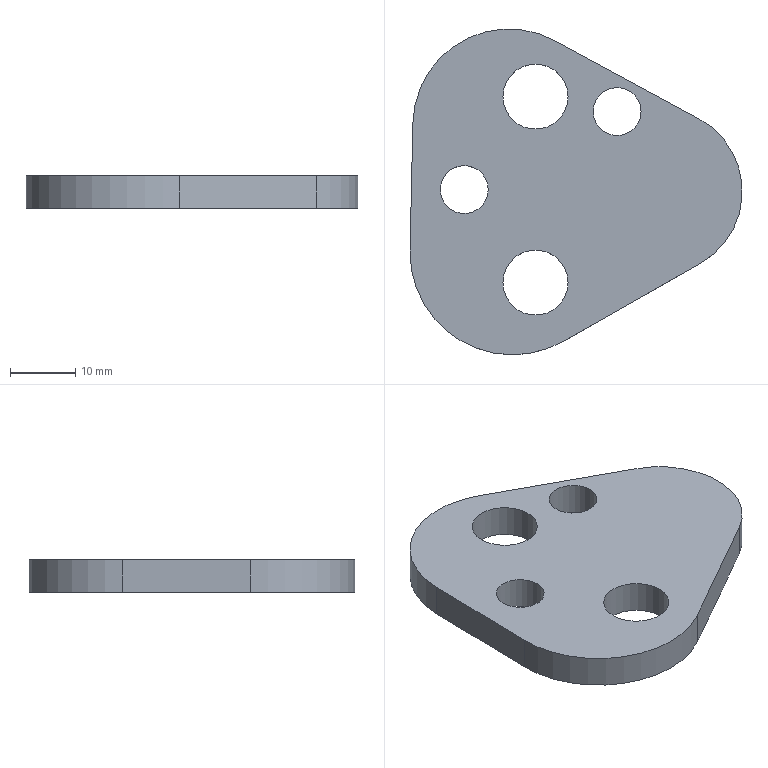Part | STEP file | 1_id198_x_t | 1 solid | 12 faces | box 51.017 x 50.028 x 5 mm | volume 8124 mm3 | cylinder 7 | plane 5 | commonest cylinder face diameters 7.35 x2 10 x2 25.4 x1 29.48 x1 31.48 x1
STEP:
#1=CARTESIAN_POINT('',(0.,0.,0.));
#2=DIRECTION('',(0.,0.,1.));
#3=DIRECTION('',(1.,0.,0.));
#4=AXIS2_PLACEMENT_3D('',#1,#2,#3);
#5=CARTESIAN_POINT('',(111.691,168.233,104.08));
#6=VERTEX_POINT('',#5);
#7=CARTESIAN_POINT('',(135.209,154.198,104.08));
#8=VERTEX_POINT('',#7);
#9=CARTESIAN_POINT('',(127.427,167.88,104.08));
#10=DIRECTION('',(0.,0.,1.));
#11=DIRECTION('',(-0.9997,0.02241,0.));
#12=AXIS2_PLACEMENT_3D('',#9,#10,#11);
#13=CIRCLE('',#12,15.74);
#14=CARTESIAN_POINT('',(127.427,167.88,109.08));
#15=DIRECTION('',(0.,0.,-1.));
#16=DIRECTION('',(1.,0.,0.));
#17=AXIS2_PLACEMENT_3D('',#14,#15,#16);
#18=CYLINDRICAL_SURFACE('',#17,15.74);
#19=CARTESIAN_POINT('',(9.447,5.));
#20=DIRECTION('',(-1.,0.));
#21=VECTOR('',#20,1.);
#22=LINE('',#19,#21);
#23=(GEOMETRIC_REPRESENTATION_CONTEXT(2)PARAMETRIC_REPRESENTATION_CONTEXT()REPRESENTATION_CONTEXT('',''));
#24=DEFINITIONAL_REPRESENTATION('',(#22),#23);
#25=PCURVE('',#18,#24);
#26=CARTESIAN_POINT('',(150.,177.5,104.08));
#27=DIRECTION('',(0.,0.,1.));
#28=DIRECTION('',(1.,0.,0.));
#29=AXIS2_PLACEMENT_3D('',#26,#27,#28);
#30=PLANE('',#29);
#31=CARTESIAN_POINT('',(-22.573,-9.62));
#32=DIRECTION('',(-0.9997,0.02241));
#33=AXIS2_PLACEMENT_2D('',#31,#32);
#34=CIRCLE('',#33,15.74);
#35=(GEOMETRIC_REPRESENTATION_CONTEXT(2)PARAMETRIC_REPRESENTATION_CONTEXT()REPRESENTATION_CONTEXT('',''));
#36=DEFINITIONAL_REPRESENTATION('',(#34),#35);
#37=PCURVE('',#30,#36);
#38=SURFACE_CURVE('',#13,(#25,#37),.PCURVE_S1.);
#39=EDGE_CURVE('',#6,#8,#38,.T.);
#40=ORIENTED_EDGE('',*,*,#39,.T.);
#41=CARTESIAN_POINT('',(135.209,154.198,109.08));
#42=VERTEX_POINT('',#41);
#43=CARTESIAN_POINT('',(135.209,154.198,104.08));
#44=DIRECTION('',(0.,0.,1.));
#45=VECTOR('',#44,1.);
#46=LINE('',#43,#45);
#47=CARTESIAN_POINT('',(1.054,5.));
#48=DIRECTION('',(0.,-1.));
#49=VECTOR('',#48,1.);
#50=LINE('',#47,#49);
#51=(GEOMETRIC_REPRESENTATION_CONTEXT(2)PARAMETRIC_REPRESENTATION_CONTEXT()REPRESENTATION_CONTEXT('',''));
#52=DEFINITIONAL_REPRESENTATION('',(#50),#51);
#53=PCURVE('',#18,#52);
#54=CARTESIAN_POINT('',(134.783,153.956,109.08));
#55=DIRECTION('',(-0.4944,0.8692,0.));
#56=DIRECTION('',(0.8692,0.4944,0.));
#57=AXIS2_PLACEMENT_3D('',#54,#55,#56);
#58=PLANE('',#57);
#59=CARTESIAN_POINT('',(0.4896,5.));
#60=DIRECTION('',(0.,-1.));
#61=VECTOR('',#60,1.);
#62=LINE('',#59,#61);
#63=(GEOMETRIC_REPRESENTATION_CONTEXT(2)PARAMETRIC_REPRESENTATION_CONTEXT()REPRESENTATION_CONTEXT('',''));
#64=DEFINITIONAL_REPRESENTATION('',(#62),#63);
#65=PCURVE('',#58,#64);
#66=SURFACE_CURVE('',#46,(#53,#65),.PCURVE_S1.);
#67=EDGE_CURVE('',#8,#42,#66,.T.);
#68=ORIENTED_EDGE('',*,*,#67,.T.);
#69=CARTESIAN_POINT('',(111.691,168.233,109.08));
#70=VERTEX_POINT('',#69);
#71=CARTESIAN_POINT('',(127.427,167.88,109.08));
#72=DIRECTION('',(0.,0.,-1.));
#73=DIRECTION('',(-1.,0.,0.));
#74=AXIS2_PLACEMENT_3D('',#71,#72,#73);
#75=CIRCLE('',#74,15.74);
#76=CARTESIAN_POINT('',(-3.142,0.));
#77=DIRECTION('',(1.,0.));
#78=VECTOR('',#77,1.);
#79=LINE('',#76,#78);
#80=(GEOMETRIC_REPRESENTATION_CONTEXT(2)PARAMETRIC_REPRESENTATION_CONTEXT()REPRESENTATION_CONTEXT('',''));
#81=DEFINITIONAL_REPRESENTATION('',(#79),#80);
#82=PCURVE('',#18,#81);
#83=CARTESIAN_POINT('',(150.,177.5,109.08));
#84=DIRECTION('',(0.,0.,1.));
#85=DIRECTION('',(1.,0.,0.));
#86=AXIS2_PLACEMENT_3D('',#83,#84,#85);
#87=PLANE('',#86);
#88=CARTESIAN_POINT('',(-38.313,-9.62));
#89=CARTESIAN_POINT('',(-38.313,17.643));
#90=CARTESIAN_POINT('',(-14.703,4.011));
#91=CARTESIAN_POINT('',(8.907,-9.62));
#92=CARTESIAN_POINT('',(-14.703,-23.251));
#93=CARTESIAN_POINT('',(-38.313,-36.882));
#94=CARTESIAN_POINT('',(-38.313,-9.62));
#95=(BOUNDED_CURVE()B_SPLINE_CURVE(2,(#88,#89,#90,#91,#92,#93,#94),.UNSPECIFIED.,.T.,.F.)B_SPLINE_CURVE_WITH_KNOTS((1,2,2,2,2,1),(-2.094,0.,2.094,4.189,6.283,8.378),.UNSPECIFIED.)CURVE()GEOMETRIC_REPRESENTATION_ITEM()RATIONAL_B_SPLINE_CURVE((1.,0.5,1.,0.5,1.,0.5,1.))REPRESENTATION_ITEM(''));
#96=(GEOMETRIC_REPRESENTATION_CONTEXT(2)PARAMETRIC_REPRESENTATION_CONTEXT()REPRESENTATION_CONTEXT('',''));
#97=DEFINITIONAL_REPRESENTATION('',(#95),#96);
#98=PCURVE('',#87,#97);
#99=SURFACE_CURVE('',#75,(#82,#98),.PCURVE_S1.);
#100=EDGE_CURVE('',#42,#70,#99,.T.);
#101=ORIENTED_EDGE('',*,*,#100,.T.);
#102=CARTESIAN_POINT('',(111.691,168.233,109.08));
#103=DIRECTION('',(0.,0.,-1.));
#104=VECTOR('',#103,1.);
#105=LINE('',#102,#104);
#106=CARTESIAN_POINT('',(3.164,0.));
#107=DIRECTION('',(0.,1.));
#108=VECTOR('',#107,1.);
#109=LINE('',#106,#108);
#110=(GEOMETRIC_REPRESENTATION_CONTEXT(2)PARAMETRIC_REPRESENTATION_CONTEXT()REPRESENTATION_CONTEXT('',''));
#111=DEFINITIONAL_REPRESENTATION('',(#109),#110);
#112=PCURVE('',#18,#111);
#113=CARTESIAN_POINT('',(112.118,187.28,109.08));
#114=DIRECTION('',(0.9997,-0.02241,0.));
#115=DIRECTION('',(0.,0.,1.));
#116=AXIS2_PLACEMENT_3D('',#113,#114,#115);
#117=PLANE('',#116);
#118=CARTESIAN_POINT('',(0.,19.052));
#119=DIRECTION('',(-1.,0.));
#120=VECTOR('',#119,1.);
#121=LINE('',#118,#120);
#122=(GEOMETRIC_REPRESENTATION_CONTEXT(2)PARAMETRIC_REPRESENTATION_CONTEXT()REPRESENTATION_CONTEXT('',''));
#123=DEFINITIONAL_REPRESENTATION('',(#121),#122);
#124=PCURVE('',#117,#123);
#125=SURFACE_CURVE('',#105,(#112,#124),.PCURVE_S1.);
#126=EDGE_CURVE('',#70,#6,#125,.T.);
#127=ORIENTED_EDGE('',*,*,#126,.T.);
#128=EDGE_LOOP('',(#40,#68,#101,#127));
#129=FACE_BOUND('',#128,.T.);
#130=ADVANCED_FACE('',(#129),#18,.T.);
#131=CARTESIAN_POINT('',(135.95,163.225,104.08));
#132=VERTEX_POINT('',#131);
#133=CARTESIAN_POINT('',(130.95,163.225,104.08));
#134=DIRECTION('',(0.,0.,1.));
#135=DIRECTION('',(1.,0.,0.));
#136=AXIS2_PLACEMENT_3D('',#133,#134,#135);
#137=CIRCLE('',#136,5.);
#138=CARTESIAN_POINT('',(-19.05,-14.275));
#139=DIRECTION('',(1.,0.));
#140=AXIS2_PLACEMENT_2D('',#138,#139);
#141=CIRCLE('',#140,5.);
#142=(GEOMETRIC_REPRESENTATION_CONTEXT(2)PARAMETRIC_REPRESENTATION_CONTEXT()REPRESENTATION_CONTEXT('',''));
#143=DEFINITIONAL_REPRESENTATION('',(#141),#142);
#144=PCURVE('',#30,#143);
#145=CARTESIAN_POINT('',(130.95,163.225,-109.08));
#146=DIRECTION('',(0.,0.,1.));
#147=DIRECTION('',(1.,0.,0.));
#148=AXIS2_PLACEMENT_3D('',#145,#146,#147);
#149=CYLINDRICAL_SURFACE('',#148,5.);
#150=CARTESIAN_POINT('',(0.,213.16));
#151=DIRECTION('',(1.,0.));
#152=VECTOR('',#151,1.);
#153=LINE('',#150,#152);
#154=(GEOMETRIC_REPRESENTATION_CONTEXT(2)PARAMETRIC_REPRESENTATION_CONTEXT()REPRESENTATION_CONTEXT('',''));
#155=DEFINITIONAL_REPRESENTATION('',(#153),#154);
#156=PCURVE('',#149,#155);
#157=SURFACE_CURVE('',#137,(#144,#156),.PCURVE_S1.);
#158=EDGE_CURVE('',#132,#132,#157,.T.);
#159=ORIENTED_EDGE('',*,*,#158,.T.);
#160=EDGE_LOOP('',(#159));
#161=FACE_BOUND('',#160,.T.);
#162=CARTESIAN_POINT('',(135.95,191.775,104.08));
#163=VERTEX_POINT('',#162);
#164=CARTESIAN_POINT('',(130.95,191.775,104.08));
#165=DIRECTION('',(0.,0.,1.));
#166=DIRECTION('',(1.,0.,0.));
#167=AXIS2_PLACEMENT_3D('',#164,#165,#166);
#168=CIRCLE('',#167,5.);
#169=CARTESIAN_POINT('',(-19.05,14.275));
#170=DIRECTION('',(1.,0.));
#171=AXIS2_PLACEMENT_2D('',#169,#170);
#172=CIRCLE('',#171,5.);
#173=(GEOMETRIC_REPRESENTATION_CONTEXT(2)PARAMETRIC_REPRESENTATION_CONTEXT()REPRESENTATION_CONTEXT('',''));
#174=DEFINITIONAL_REPRESENTATION('',(#172),#173);
#175=PCURVE('',#30,#174);
#176=CARTESIAN_POINT('',(130.95,191.775,-109.08));
#177=DIRECTION('',(0.,0.,1.));
#178=DIRECTION('',(1.,0.,0.));
#179=AXIS2_PLACEMENT_3D('',#176,#177,#178);
#180=CYLINDRICAL_SURFACE('',#179,5.);
#181=CARTESIAN_POINT('',(0.,213.16));
#182=DIRECTION('',(1.,0.));
#183=VECTOR('',#182,1.);
#184=LINE('',#181,#183);
#185=(GEOMETRIC_REPRESENTATION_CONTEXT(2)PARAMETRIC_REPRESENTATION_CONTEXT()REPRESENTATION_CONTEXT('',''));
#186=DEFINITIONAL_REPRESENTATION('',(#184),#185);
#187=PCURVE('',#180,#186);
#188=SURFACE_CURVE('',#168,(#175,#187),.PCURVE_S1.);
#189=EDGE_CURVE('',#163,#163,#188,.T.);
#190=ORIENTED_EDGE('',*,*,#189,.T.);
#191=EDGE_LOOP('',(#190));
#192=FACE_BOUND('',#191,.T.);
#193=ORIENTED_EDGE('',*,*,#39,.F.);
#194=CARTESIAN_POINT('',(112.129,187.758,104.08));
#195=VERTEX_POINT('',#194);
#196=CARTESIAN_POINT('',(111.918,178.354,104.08));
#197=DIRECTION('',(0.02241,0.9997,0.));
#198=VECTOR('',#197,1.);
#199=LINE('',#196,#198);
#200=CARTESIAN_POINT('',(-38.082,0.8537));
#201=DIRECTION('',(0.02241,0.9997));
#202=VECTOR('',#201,1.);
#203=LINE('',#200,#202);
#204=(GEOMETRIC_REPRESENTATION_CONTEXT(2)PARAMETRIC_REPRESENTATION_CONTEXT()REPRESENTATION_CONTEXT('',''));
#205=DEFINITIONAL_REPRESENTATION('',(#203),#204);
#206=PCURVE('',#30,#205);
#207=CARTESIAN_POINT('',(-5.,8.928));
#208=DIRECTION('',(0.,-1.));
#209=VECTOR('',#208,1.);
#210=LINE('',#207,#209);
#211=(GEOMETRIC_REPRESENTATION_CONTEXT(2)PARAMETRIC_REPRESENTATION_CONTEXT()REPRESENTATION_CONTEXT('',''));
#212=DEFINITIONAL_REPRESENTATION('',(#210),#211);
#213=PCURVE('',#117,#212);
#214=SURFACE_CURVE('',#199,(#206,#213),.PCURVE_S1.);
#215=EDGE_CURVE('',#6,#195,#214,.T.);
#216=ORIENTED_EDGE('',*,*,#215,.T.);
#217=CARTESIAN_POINT('',(133.881,200.391,104.08));
#218=VERTEX_POINT('',#217);
#219=CARTESIAN_POINT('',(126.865,187.428,104.08));
#220=DIRECTION('',(0.,0.,-1.));
#221=DIRECTION('',(-0.9997,0.02241,0.));
#222=AXIS2_PLACEMENT_3D('',#219,#220,#221);
#223=CIRCLE('',#222,14.74);
#224=CARTESIAN_POINT('',(-37.871,10.258));
#225=CARTESIAN_POINT('',(-37.299,35.782));
#226=CARTESIAN_POINT('',(-15.481,22.525));
#227=CARTESIAN_POINT('',(6.338,9.267));
#228=CARTESIAN_POINT('',(-16.053,-2.999));
#229=CARTESIAN_POINT('',(-38.444,-15.266));
#230=CARTESIAN_POINT('',(-37.871,10.258));
#231=(BOUNDED_CURVE()B_SPLINE_CURVE(2,(#224,#225,#226,#227,#228,#229,#230),.UNSPECIFIED.,.T.,.F.)B_SPLINE_CURVE_WITH_KNOTS((1,2,2,2,2,1),(-2.094,0.,2.094,4.189,6.283,8.378),.UNSPECIFIED.)CURVE()GEOMETRIC_REPRESENTATION_ITEM()RATIONAL_B_SPLINE_CURVE((1.,0.5,1.,0.5,1.,0.5,1.))REPRESENTATION_ITEM(''));
#232=(GEOMETRIC_REPRESENTATION_CONTEXT(2)PARAMETRIC_REPRESENTATION_CONTEXT()REPRESENTATION_CONTEXT('',''));
#233=DEFINITIONAL_REPRESENTATION('',(#231),#232);
#234=PCURVE('',#30,#233);
#235=CARTESIAN_POINT('',(126.865,187.428,109.08));
#236=DIRECTION('',(0.,0.,-1.));
#237=DIRECTION('',(1.,0.,0.));
#238=AXIS2_PLACEMENT_3D('',#235,#236,#237);
#239=CYLINDRICAL_SURFACE('',#238,14.74);
#240=CARTESIAN_POINT('',(3.164,5.));
#241=DIRECTION('',(1.,0.));
#242=VECTOR('',#241,1.);
#243=LINE('',#240,#242);
#244=(GEOMETRIC_REPRESENTATION_CONTEXT(2)PARAMETRIC_REPRESENTATION_CONTEXT()REPRESENTATION_CONTEXT('',''));
#245=DEFINITIONAL_REPRESENTATION('',(#243),#244);
#246=PCURVE('',#239,#245);
#247=SURFACE_CURVE('',#223,(#234,#246),.PCURVE_S1.);
#248=EDGE_CURVE('',#195,#218,#247,.T.);
#249=ORIENTED_EDGE('',*,*,#248,.T.);
#250=CARTESIAN_POINT('',(156.049,188.393,104.08));
#251=VERTEX_POINT('',#250);
#252=CARTESIAN_POINT('',(133.881,200.391,104.08));
#253=DIRECTION('',(0.8795,-0.476,0.));
#254=VECTOR('',#253,1.);
#255=LINE('',#252,#254);
#256=CARTESIAN_POINT('',(-16.119,22.891));
#257=DIRECTION('',(0.8795,-0.476));
#258=VECTOR('',#257,1.);
#259=LINE('',#256,#258);
#260=(GEOMETRIC_REPRESENTATION_CONTEXT(2)PARAMETRIC_REPRESENTATION_CONTEXT()REPRESENTATION_CONTEXT('',''));
#261=DEFINITIONAL_REPRESENTATION('',(#259),#260);
#262=PCURVE('',#30,#261);
#263=CARTESIAN_POINT('',(156.047,188.394,109.08));
#264=DIRECTION('',(-0.476,-0.8795,0.));
#265=DIRECTION('',(-0.8795,0.476,0.));
#266=AXIS2_PLACEMENT_3D('',#263,#264,#265);
#267=PLANE('',#266);
#268=CARTESIAN_POINT('',(25.205,5.));
#269=DIRECTION('',(-1.,0.));
#270=VECTOR('',#269,1.);
#271=LINE('',#268,#270);
#272=(GEOMETRIC_REPRESENTATION_CONTEXT(2)PARAMETRIC_REPRESENTATION_CONTEXT()REPRESENTATION_CONTEXT('',''));
#273=DEFINITIONAL_REPRESENTATION('',(#271),#272);
#274=PCURVE('',#267,#273);
#275=SURFACE_CURVE('',#255,(#262,#274),.PCURVE_S1.);
#276=EDGE_CURVE('',#218,#251,#275,.T.);
#277=ORIENTED_EDGE('',*,*,#276,.T.);
#278=CARTESIAN_POINT('',(156.283,166.185,104.08));
#279=VERTEX_POINT('',#278);
#280=CARTESIAN_POINT('',(150.004,177.224,104.08));
#281=DIRECTION('',(0.,0.,-1.));
#282=DIRECTION('',(1.,0.,0.));
#283=AXIS2_PLACEMENT_3D('',#280,#281,#282);
#284=CIRCLE('',#283,12.7);
#285=CARTESIAN_POINT('',(12.704,-0.2758));
#286=CARTESIAN_POINT('',(12.704,-22.273));
#287=CARTESIAN_POINT('',(-6.346,-11.274));
#288=CARTESIAN_POINT('',(-25.396,-0.2758));
#289=CARTESIAN_POINT('',(-6.346,10.723));
#290=CARTESIAN_POINT('',(12.704,21.721));
#291=CARTESIAN_POINT('',(12.704,-0.2758));
#292=(BOUNDED_CURVE()B_SPLINE_CURVE(2,(#285,#286,#287,#288,#289,#290,#291),.UNSPECIFIED.,.T.,.F.)B_SPLINE_CURVE_WITH_KNOTS((1,2,2,2,2,1),(-2.094,0.,2.094,4.189,6.283,8.378),.UNSPECIFIED.)CURVE()GEOMETRIC_REPRESENTATION_ITEM()RATIONAL_B_SPLINE_CURVE((1.,0.5,1.,0.5,1.,0.5,1.))REPRESENTATION_ITEM(''));
#293=(GEOMETRIC_REPRESENTATION_CONTEXT(2)PARAMETRIC_REPRESENTATION_CONTEXT()REPRESENTATION_CONTEXT('',''));
#294=DEFINITIONAL_REPRESENTATION('',(#292),#293);
#295=PCURVE('',#30,#294);
#296=CARTESIAN_POINT('',(150.004,177.224,109.08));
#297=DIRECTION('',(0.,0.,-1.));
#298=DIRECTION('',(1.,0.,0.));
#299=AXIS2_PLACEMENT_3D('',#296,#297,#298);
#300=CYLINDRICAL_SURFACE('',#299,12.7);
#301=CARTESIAN_POINT('',(0.,5.));
#302=DIRECTION('',(1.,0.));
#303=VECTOR('',#302,1.);
#304=LINE('',#301,#303);
#305=(GEOMETRIC_REPRESENTATION_CONTEXT(2)PARAMETRIC_REPRESENTATION_CONTEXT()REPRESENTATION_CONTEXT('',''));
#306=DEFINITIONAL_REPRESENTATION('',(#304),#305);
#307=PCURVE('',#300,#306);
#308=SURFACE_CURVE('',#284,(#295,#307),.PCURVE_S1.);
#309=EDGE_CURVE('',#251,#279,#308,.T.);
#310=ORIENTED_EDGE('',*,*,#309,.T.);
#311=CARTESIAN_POINT('',(156.283,166.185,104.08));
#312=DIRECTION('',(-0.8692,-0.4944,0.));
#313=VECTOR('',#312,1.);
#314=LINE('',#311,#313);
#315=CARTESIAN_POINT('',(6.283,-11.315));
#316=DIRECTION('',(-0.8692,-0.4944));
#317=VECTOR('',#316,1.);
#318=LINE('',#315,#317);
#319=(GEOMETRIC_REPRESENTATION_CONTEXT(2)PARAMETRIC_REPRESENTATION_CONTEXT()REPRESENTATION_CONTEXT('',''));
#320=DEFINITIONAL_REPRESENTATION('',(#318),#319);
#321=PCURVE('',#30,#320);
#322=CARTESIAN_POINT('',(24.734,5.));
#323=DIRECTION('',(-1.,0.));
#324=VECTOR('',#323,1.);
#325=LINE('',#322,#324);
#326=(GEOMETRIC_REPRESENTATION_CONTEXT(2)PARAMETRIC_REPRESENTATION_CONTEXT()REPRESENTATION_CONTEXT('',''));
#327=DEFINITIONAL_REPRESENTATION('',(#325),#326);
#328=PCURVE('',#58,#327);
#329=SURFACE_CURVE('',#314,(#321,#328),.PCURVE_S1.);
#330=EDGE_CURVE('',#279,#8,#329,.T.);
#331=ORIENTED_EDGE('',*,*,#330,.T.);
#332=EDGE_LOOP('',(#193,#216,#249,#277,#310,#331));
#333=FACE_BOUND('',#332,.T.);
#334=CARTESIAN_POINT('',(147.173,189.489,104.08));
#335=VERTEX_POINT('',#334);
#336=CARTESIAN_POINT('',(143.498,189.489,104.08));
#337=DIRECTION('',(0.,0.,1.));
#338=DIRECTION('',(1.,0.,0.));
#339=AXIS2_PLACEMENT_3D('',#336,#337,#338);
#340=CIRCLE('',#339,3.675);
#341=CARTESIAN_POINT('',(-6.502,11.989));
#342=DIRECTION('',(1.,0.));
#343=AXIS2_PLACEMENT_2D('',#341,#342);
#344=CIRCLE('',#343,3.675);
#345=(GEOMETRIC_REPRESENTATION_CONTEXT(2)PARAMETRIC_REPRESENTATION_CONTEXT()REPRESENTATION_CONTEXT('',''));
#346=DEFINITIONAL_REPRESENTATION('',(#344),#345);
#347=PCURVE('',#30,#346);
#348=CARTESIAN_POINT('',(143.498,189.489,109.08));
#349=DIRECTION('',(0.,0.,-1.));
#350=DIRECTION('',(1.,0.,0.));
#351=AXIS2_PLACEMENT_3D('',#348,#349,#350);
#352=CYLINDRICAL_SURFACE('',#351,3.675);
#353=CARTESIAN_POINT('',(6.283,5.));
#354=DIRECTION('',(-1.,0.));
#355=VECTOR('',#354,1.);
#356=LINE('',#353,#355);
#357=(GEOMETRIC_REPRESENTATION_CONTEXT(2)PARAMETRIC_REPRESENTATION_CONTEXT()REPRESENTATION_CONTEXT('',''));
#358=DEFINITIONAL_REPRESENTATION('',(#356),#357);
#359=PCURVE('',#352,#358);
#360=SURFACE_CURVE('',#340,(#347,#359),.PCURVE_S1.);
#361=EDGE_CURVE('',#335,#335,#360,.T.);
#362=ORIENTED_EDGE('',*,*,#361,.T.);
#363=EDGE_LOOP('',(#362));
#364=FACE_BOUND('',#363,.T.);
#365=CARTESIAN_POINT('',(123.703,177.5,104.08));
#366=VERTEX_POINT('',#365);
#367=CARTESIAN_POINT('',(120.028,177.5,104.08));
#368=DIRECTION('',(0.,0.,1.));
#369=DIRECTION('',(1.,0.,0.));
#370=AXIS2_PLACEMENT_3D('',#367,#368,#369);
#371=CIRCLE('',#370,3.675);
#372=CARTESIAN_POINT('',(-29.972,0.));
#373=DIRECTION('',(1.,0.));
#374=AXIS2_PLACEMENT_2D('',#372,#373);
#375=CIRCLE('',#374,3.675);
#376=(GEOMETRIC_REPRESENTATION_CONTEXT(2)PARAMETRIC_REPRESENTATION_CONTEXT()REPRESENTATION_CONTEXT('',''));
#377=DEFINITIONAL_REPRESENTATION('',(#375),#376);
#378=PCURVE('',#30,#377);
#379=CARTESIAN_POINT('',(120.028,177.5,109.08));
#380=DIRECTION('',(0.,0.,-1.));
#381=DIRECTION('',(1.,0.,0.));
#382=AXIS2_PLACEMENT_3D('',#379,#380,#381);
#383=CYLINDRICAL_SURFACE('',#382,3.675);
#384=CARTESIAN_POINT('',(6.283,5.));
#385=DIRECTION('',(-1.,0.));
#386=VECTOR('',#385,1.);
#387=LINE('',#384,#386);
#388=(GEOMETRIC_REPRESENTATION_CONTEXT(2)PARAMETRIC_REPRESENTATION_CONTEXT()REPRESENTATION_CONTEXT('',''));
#389=DEFINITIONAL_REPRESENTATION('',(#387),#388);
#390=PCURVE('',#383,#389);
#391=SURFACE_CURVE('',#371,(#378,#390),.PCURVE_S1.);
#392=EDGE_CURVE('',#366,#366,#391,.T.);
#393=ORIENTED_EDGE('',*,*,#392,.T.);
#394=EDGE_LOOP('',(#393));
#395=FACE_BOUND('',#394,.T.);
#396=ADVANCED_FACE('',(#161,#192,#333,#364,#395),#30,.F.);
#397=CARTESIAN_POINT('',(156.283,166.185,109.08));
#398=VERTEX_POINT('',#397);
#399=CARTESIAN_POINT('',(156.283,166.185,109.08));
#400=DIRECTION('',(0.,0.,-1.));
#401=VECTOR('',#400,1.);
#402=LINE('',#399,#401);
#403=CARTESIAN_POINT('',(24.734,0.));
#404=DIRECTION('',(0.,1.));
#405=VECTOR('',#404,1.);
#406=LINE('',#403,#405);
#407=(GEOMETRIC_REPRESENTATION_CONTEXT(2)PARAMETRIC_REPRESENTATION_CONTEXT()REPRESENTATION_CONTEXT('',''));
#408=DEFINITIONAL_REPRESENTATION('',(#406),#407);
#409=PCURVE('',#58,#408);
#410=CARTESIAN_POINT('',(7.337,0.));
#411=DIRECTION('',(0.,1.));
#412=VECTOR('',#411,1.);
#413=LINE('',#410,#412);
#414=(GEOMETRIC_REPRESENTATION_CONTEXT(2)PARAMETRIC_REPRESENTATION_CONTEXT()REPRESENTATION_CONTEXT('',''));
#415=DEFINITIONAL_REPRESENTATION('',(#413),#414);
#416=PCURVE('',#300,#415);
#417=SURFACE_CURVE('',#402,(#409,#416),.PCURVE_S1.);
#418=EDGE_CURVE('',#398,#279,#417,.T.);
#419=ORIENTED_EDGE('',*,*,#418,.F.);
#420=CARTESIAN_POINT('',(135.209,154.198,109.08));
#421=DIRECTION('',(0.8692,0.4944,0.));
#422=VECTOR('',#421,1.);
#423=LINE('',#420,#422);
#424=CARTESIAN_POINT('',(0.4896,0.));
#425=DIRECTION('',(1.,0.));
#426=VECTOR('',#425,1.);
#427=LINE('',#424,#426);
#428=(GEOMETRIC_REPRESENTATION_CONTEXT(2)PARAMETRIC_REPRESENTATION_CONTEXT()REPRESENTATION_CONTEXT('',''));
#429=DEFINITIONAL_REPRESENTATION('',(#427),#428);
#430=PCURVE('',#58,#429);
#431=CARTESIAN_POINT('',(-14.791,-23.302));
#432=DIRECTION('',(0.8692,0.4944));
#433=VECTOR('',#432,1.);
#434=LINE('',#431,#433);
#435=(GEOMETRIC_REPRESENTATION_CONTEXT(2)PARAMETRIC_REPRESENTATION_CONTEXT()REPRESENTATION_CONTEXT('',''));
#436=DEFINITIONAL_REPRESENTATION('',(#434),#435);
#437=PCURVE('',#87,#436);
#438=SURFACE_CURVE('',#423,(#430,#437),.PCURVE_S1.);
#439=EDGE_CURVE('',#42,#398,#438,.T.);
#440=ORIENTED_EDGE('',*,*,#439,.F.);
#441=ORIENTED_EDGE('',*,*,#67,.F.);
#442=ORIENTED_EDGE('',*,*,#330,.F.);
#443=EDGE_LOOP('',(#419,#440,#441,#442));
#444=FACE_BOUND('',#443,.T.);
#445=ADVANCED_FACE('',(#444),#58,.F.);
#446=CARTESIAN_POINT('',(135.95,163.225,109.08));
#447=VERTEX_POINT('',#446);
#448=CARTESIAN_POINT('',(130.95,163.225,109.08));
#449=DIRECTION('',(0.,0.,1.));
#450=DIRECTION('',(1.,0.,0.));
#451=AXIS2_PLACEMENT_3D('',#448,#449,#450);
#452=CIRCLE('',#451,5.);
#453=CARTESIAN_POINT('',(-19.05,-14.275));
#454=DIRECTION('',(1.,0.));
#455=AXIS2_PLACEMENT_2D('',#453,#454);
#456=CIRCLE('',#455,5.);
#457=(GEOMETRIC_REPRESENTATION_CONTEXT(2)PARAMETRIC_REPRESENTATION_CONTEXT()REPRESENTATION_CONTEXT('',''));
#458=DEFINITIONAL_REPRESENTATION('',(#456),#457);
#459=PCURVE('',#87,#458);
#460=CARTESIAN_POINT('',(0.,218.16));
#461=DIRECTION('',(1.,0.));
#462=VECTOR('',#461,1.);
#463=LINE('',#460,#462);
#464=(GEOMETRIC_REPRESENTATION_CONTEXT(2)PARAMETRIC_REPRESENTATION_CONTEXT()REPRESENTATION_CONTEXT('',''));
#465=DEFINITIONAL_REPRESENTATION('',(#463),#464);
#466=PCURVE('',#149,#465);
#467=SURFACE_CURVE('',#452,(#459,#466),.PCURVE_S1.);
#468=EDGE_CURVE('',#447,#447,#467,.T.);
#469=ORIENTED_EDGE('',*,*,#468,.F.);
#470=EDGE_LOOP('',(#469));
#471=FACE_BOUND('',#470,.T.);
#472=CARTESIAN_POINT('',(135.95,191.775,109.08));
#473=VERTEX_POINT('',#472);
#474=CARTESIAN_POINT('',(130.95,191.775,109.08));
#475=DIRECTION('',(0.,0.,1.));
#476=DIRECTION('',(1.,0.,0.));
#477=AXIS2_PLACEMENT_3D('',#474,#475,#476);
#478=CIRCLE('',#477,5.);
#479=CARTESIAN_POINT('',(-19.05,14.275));
#480=DIRECTION('',(1.,0.));
#481=AXIS2_PLACEMENT_2D('',#479,#480);
#482=CIRCLE('',#481,5.);
#483=(GEOMETRIC_REPRESENTATION_CONTEXT(2)PARAMETRIC_REPRESENTATION_CONTEXT()REPRESENTATION_CONTEXT('',''));
#484=DEFINITIONAL_REPRESENTATION('',(#482),#483);
#485=PCURVE('',#87,#484);
#486=CARTESIAN_POINT('',(0.,218.16));
#487=DIRECTION('',(1.,0.));
#488=VECTOR('',#487,1.);
#489=LINE('',#486,#488);
#490=(GEOMETRIC_REPRESENTATION_CONTEXT(2)PARAMETRIC_REPRESENTATION_CONTEXT()REPRESENTATION_CONTEXT('',''));
#491=DEFINITIONAL_REPRESENTATION('',(#489),#490);
#492=PCURVE('',#180,#491);
#493=SURFACE_CURVE('',#478,(#485,#492),.PCURVE_S1.);
#494=EDGE_CURVE('',#473,#473,#493,.T.);
#495=ORIENTED_EDGE('',*,*,#494,.F.);
#496=EDGE_LOOP('',(#495));
#497=FACE_BOUND('',#496,.T.);
#498=ORIENTED_EDGE('',*,*,#100,.F.);
#499=ORIENTED_EDGE('',*,*,#439,.T.);
#500=CARTESIAN_POINT('',(156.049,188.393,109.08));
#501=VERTEX_POINT('',#500);
#502=CARTESIAN_POINT('',(150.004,177.224,109.08));
#503=DIRECTION('',(0.,0.,1.));
#504=DIRECTION('',(1.,0.,0.));
#505=AXIS2_PLACEMENT_3D('',#502,#503,#504);
#506=CIRCLE('',#505,12.7);
#507=CARTESIAN_POINT('',(0.004012,-0.2758));
#508=DIRECTION('',(1.,0.));
#509=AXIS2_PLACEMENT_2D('',#507,#508);
#510=CIRCLE('',#509,12.7);
#511=(GEOMETRIC_REPRESENTATION_CONTEXT(2)PARAMETRIC_REPRESENTATION_CONTEXT()REPRESENTATION_CONTEXT('',''));
#512=DEFINITIONAL_REPRESENTATION('',(#510),#511);
#513=PCURVE('',#87,#512);
#514=CARTESIAN_POINT('',(12.566,0.));
#515=DIRECTION('',(-1.,0.));
#516=VECTOR('',#515,1.);
#517=LINE('',#514,#516);
#518=(GEOMETRIC_REPRESENTATION_CONTEXT(2)PARAMETRIC_REPRESENTATION_CONTEXT()REPRESENTATION_CONTEXT('',''));
#519=DEFINITIONAL_REPRESENTATION('',(#517),#518);
#520=PCURVE('',#300,#519);
#521=SURFACE_CURVE('',#506,(#513,#520),.PCURVE_S1.);
#522=EDGE_CURVE('',#398,#501,#521,.T.);
#523=ORIENTED_EDGE('',*,*,#522,.T.);
#524=CARTESIAN_POINT('',(133.881,200.391,109.08));
#525=VERTEX_POINT('',#524);
#526=CARTESIAN_POINT('',(156.049,188.393,109.08));
#527=DIRECTION('',(-0.8795,0.476,0.));
#528=VECTOR('',#527,1.);
#529=LINE('',#526,#528);
#530=CARTESIAN_POINT('',(6.049,10.893));
#531=DIRECTION('',(-0.8795,0.476));
#532=VECTOR('',#531,1.);
#533=LINE('',#530,#532);
#534=(GEOMETRIC_REPRESENTATION_CONTEXT(2)PARAMETRIC_REPRESENTATION_CONTEXT()REPRESENTATION_CONTEXT('',''));
#535=DEFINITIONAL_REPRESENTATION('',(#533),#534);
#536=PCURVE('',#87,#535);
#537=CARTESIAN_POINT('',(-0.001671,0.));
#538=DIRECTION('',(1.,0.));
#539=VECTOR('',#538,1.);
#540=LINE('',#537,#539);
#541=(GEOMETRIC_REPRESENTATION_CONTEXT(2)PARAMETRIC_REPRESENTATION_CONTEXT()REPRESENTATION_CONTEXT('',''));
#542=DEFINITIONAL_REPRESENTATION('',(#540),#541);
#543=PCURVE('',#267,#542);
#544=SURFACE_CURVE('',#529,(#536,#543),.PCURVE_S1.);
#545=EDGE_CURVE('',#501,#525,#544,.T.);
#546=ORIENTED_EDGE('',*,*,#545,.T.);
#547=CARTESIAN_POINT('',(112.129,187.758,109.08));
#548=VERTEX_POINT('',#547);
#549=CARTESIAN_POINT('',(126.865,187.428,109.08));
#550=DIRECTION('',(0.,0.,1.));
#551=DIRECTION('',(0.476,0.8795,0.));
#552=AXIS2_PLACEMENT_3D('',#549,#550,#551);
#553=CIRCLE('',#552,14.74);
#554=CARTESIAN_POINT('',(-23.135,9.928));
#555=DIRECTION('',(0.476,0.8795));
#556=AXIS2_PLACEMENT_2D('',#554,#555);
#557=CIRCLE('',#556,14.74);
#558=(GEOMETRIC_REPRESENTATION_CONTEXT(2)PARAMETRIC_REPRESENTATION_CONTEXT()REPRESENTATION_CONTEXT('',''));
#559=DEFINITIONAL_REPRESENTATION('',(#557),#558);
#560=PCURVE('',#87,#559);
#561=CARTESIAN_POINT('',(5.208,0.));
#562=DIRECTION('',(-1.,0.));
#563=VECTOR('',#562,1.);
#564=LINE('',#561,#563);
#565=(GEOMETRIC_REPRESENTATION_CONTEXT(2)PARAMETRIC_REPRESENTATION_CONTEXT()REPRESENTATION_CONTEXT('',''));
#566=DEFINITIONAL_REPRESENTATION('',(#564),#565);
#567=PCURVE('',#239,#566);
#568=SURFACE_CURVE('',#553,(#560,#567),.PCURVE_S1.);
#569=EDGE_CURVE('',#525,#548,#568,.T.);
#570=ORIENTED_EDGE('',*,*,#569,.T.);
#571=CARTESIAN_POINT('',(112.118,187.28,109.08));
#572=DIRECTION('',(-0.02241,-0.9997,0.));
#573=VECTOR('',#572,1.);
#574=LINE('',#571,#573);
#575=CARTESIAN_POINT('',(-37.882,9.78));
#576=DIRECTION('',(-0.02241,-0.9997));
#577=VECTOR('',#576,1.);
#578=LINE('',#575,#577);
#579=(GEOMETRIC_REPRESENTATION_CONTEXT(2)PARAMETRIC_REPRESENTATION_CONTEXT()REPRESENTATION_CONTEXT('',''));
#580=DEFINITIONAL_REPRESENTATION('',(#578),#579);
#581=PCURVE('',#87,#580);
#582=CARTESIAN_POINT('',(0.,0.));
#583=DIRECTION('',(0.,1.));
#584=VECTOR('',#583,1.);
#585=LINE('',#582,#584);
#586=(GEOMETRIC_REPRESENTATION_CONTEXT(2)PARAMETRIC_REPRESENTATION_CONTEXT()REPRESENTATION_CONTEXT('',''));
#587=DEFINITIONAL_REPRESENTATION('',(#585),#586);
#588=PCURVE('',#117,#587);
#589=SURFACE_CURVE('',#574,(#581,#588),.PCURVE_S1.);
#590=EDGE_CURVE('',#548,#70,#589,.T.);
#591=ORIENTED_EDGE('',*,*,#590,.T.);
#592=EDGE_LOOP('',(#498,#499,#523,#546,#570,#591));
#593=FACE_BOUND('',#592,.T.);
#594=CARTESIAN_POINT('',(147.173,189.489,109.08));
#595=VERTEX_POINT('',#594);
#596=CARTESIAN_POINT('',(143.498,189.489,109.08));
#597=DIRECTION('',(0.,0.,-1.));
#598=DIRECTION('',(1.,0.,0.));
#599=AXIS2_PLACEMENT_3D('',#596,#597,#598);
#600=CIRCLE('',#599,3.675);
#601=CARTESIAN_POINT('',(-2.827,11.989));
#602=CARTESIAN_POINT('',(-2.827,5.624));
#603=CARTESIAN_POINT('',(-8.34,8.806));
#604=CARTESIAN_POINT('',(-13.852,11.989));
#605=CARTESIAN_POINT('',(-8.34,15.171));
#606=CARTESIAN_POINT('',(-2.827,18.354));
#607=CARTESIAN_POINT('',(-2.827,11.989));
#608=(BOUNDED_CURVE()B_SPLINE_CURVE(2,(#601,#602,#603,#604,#605,#606,#607),.UNSPECIFIED.,.T.,.F.)B_SPLINE_CURVE_WITH_KNOTS((1,2,2,2,2,1),(-2.094,0.,2.094,4.189,6.283,8.378),.UNSPECIFIED.)CURVE()GEOMETRIC_REPRESENTATION_ITEM()RATIONAL_B_SPLINE_CURVE((1.,0.5,1.,0.5,1.,0.5,1.))REPRESENTATION_ITEM(''));
#609=(GEOMETRIC_REPRESENTATION_CONTEXT(2)PARAMETRIC_REPRESENTATION_CONTEXT()REPRESENTATION_CONTEXT('',''));
#610=DEFINITIONAL_REPRESENTATION('',(#608),#609);
#611=PCURVE('',#87,#610);
#612=CARTESIAN_POINT('',(0.,0.));
#613=DIRECTION('',(1.,0.));
#614=VECTOR('',#613,1.);
#615=LINE('',#612,#614);
#616=(GEOMETRIC_REPRESENTATION_CONTEXT(2)PARAMETRIC_REPRESENTATION_CONTEXT()REPRESENTATION_CONTEXT('',''));
#617=DEFINITIONAL_REPRESENTATION('',(#615),#616);
#618=PCURVE('',#352,#617);
#619=SURFACE_CURVE('',#600,(#611,#618),.PCURVE_S1.);
#620=EDGE_CURVE('',#595,#595,#619,.T.);
#621=ORIENTED_EDGE('',*,*,#620,.T.);
#622=EDGE_LOOP('',(#621));
#623=FACE_BOUND('',#622,.T.);
#624=CARTESIAN_POINT('',(123.703,177.5,109.08));
#625=VERTEX_POINT('',#624);
#626=CARTESIAN_POINT('',(120.028,177.5,109.08));
#627=DIRECTION('',(0.,0.,-1.));
#628=DIRECTION('',(1.,0.,0.));
#629=AXIS2_PLACEMENT_3D('',#626,#627,#628);
#630=CIRCLE('',#629,3.675);
#631=CARTESIAN_POINT('',(-26.297,0.));
#632=CARTESIAN_POINT('',(-26.297,-6.365));
#633=CARTESIAN_POINT('',(-31.809,-3.183));
#634=CARTESIAN_POINT('',(-37.322,0.));
#635=CARTESIAN_POINT('',(-31.809,3.183));
#636=CARTESIAN_POINT('',(-26.297,6.365));
#637=CARTESIAN_POINT('',(-26.297,0.));
#638=(BOUNDED_CURVE()B_SPLINE_CURVE(2,(#631,#632,#633,#634,#635,#636,#637),.UNSPECIFIED.,.T.,.F.)B_SPLINE_CURVE_WITH_KNOTS((1,2,2,2,2,1),(-2.094,0.,2.094,4.189,6.283,8.378),.UNSPECIFIED.)CURVE()GEOMETRIC_REPRESENTATION_ITEM()RATIONAL_B_SPLINE_CURVE((1.,0.5,1.,0.5,1.,0.5,1.))REPRESENTATION_ITEM(''));
#639=(GEOMETRIC_REPRESENTATION_CONTEXT(2)PARAMETRIC_REPRESENTATION_CONTEXT()REPRESENTATION_CONTEXT('',''));
#640=DEFINITIONAL_REPRESENTATION('',(#638),#639);
#641=PCURVE('',#87,#640);
#642=CARTESIAN_POINT('',(0.,0.));
#643=DIRECTION('',(1.,0.));
#644=VECTOR('',#643,1.);
#645=LINE('',#642,#644);
#646=(GEOMETRIC_REPRESENTATION_CONTEXT(2)PARAMETRIC_REPRESENTATION_CONTEXT()REPRESENTATION_CONTEXT('',''));
#647=DEFINITIONAL_REPRESENTATION('',(#645),#646);
#648=PCURVE('',#383,#647);
#649=SURFACE_CURVE('',#630,(#641,#648),.PCURVE_S1.);
#650=EDGE_CURVE('',#625,#625,#649,.T.);
#651=ORIENTED_EDGE('',*,*,#650,.T.);
#652=EDGE_LOOP('',(#651));
#653=FACE_BOUND('',#652,.T.);
#654=ADVANCED_FACE('',(#471,#497,#593,#623,#653),#87,.T.);
#655=ORIENTED_EDGE('',*,*,#126,.F.);
#656=ORIENTED_EDGE('',*,*,#590,.F.);
#657=CARTESIAN_POINT('',(112.129,187.758,104.08));
#658=DIRECTION('',(0.,0.,1.));
#659=VECTOR('',#658,1.);
#660=LINE('',#657,#659);
#661=CARTESIAN_POINT('',(-5.,-0.4785));
#662=DIRECTION('',(1.,0.));
#663=VECTOR('',#662,1.);
#664=LINE('',#661,#663);
#665=(GEOMETRIC_REPRESENTATION_CONTEXT(2)PARAMETRIC_REPRESENTATION_CONTEXT()REPRESENTATION_CONTEXT('',''));
#666=DEFINITIONAL_REPRESENTATION('',(#664),#665);
#667=PCURVE('',#117,#666);
#668=CARTESIAN_POINT('',(3.164,5.));
#669=DIRECTION('',(0.,-1.));
#670=VECTOR('',#669,1.);
#671=LINE('',#668,#670);
#672=(GEOMETRIC_REPRESENTATION_CONTEXT(2)PARAMETRIC_REPRESENTATION_CONTEXT()REPRESENTATION_CONTEXT('',''));
#673=DEFINITIONAL_REPRESENTATION('',(#671),#672);
#674=PCURVE('',#239,#673);
#675=SURFACE_CURVE('',#660,(#667,#674),.PCURVE_S1.);
#676=EDGE_CURVE('',#195,#548,#675,.T.);
#677=ORIENTED_EDGE('',*,*,#676,.F.);
#678=ORIENTED_EDGE('',*,*,#215,.F.);
#679=EDGE_LOOP('',(#655,#656,#677,#678));
#680=FACE_BOUND('',#679,.T.);
#681=ADVANCED_FACE('',(#680),#117,.F.);
#682=ORIENTED_EDGE('',*,*,#676,.T.);
#683=ORIENTED_EDGE('',*,*,#569,.F.);
#684=CARTESIAN_POINT('',(133.881,200.391,109.08));
#685=DIRECTION('',(-0.000000278,0.00000015,-1.));
#686=VECTOR('',#685,1.);
#687=LINE('',#684,#686);
#688=CARTESIAN_POINT('',(5.208,0.));
#689=DIRECTION('',(-0.000000021,1.));
#690=VECTOR('',#689,1.);
#691=LINE('',#688,#690);
#692=(GEOMETRIC_REPRESENTATION_CONTEXT(2)PARAMETRIC_REPRESENTATION_CONTEXT()REPRESENTATION_CONTEXT('',''));
#693=DEFINITIONAL_REPRESENTATION('',(#691),#692);
#694=PCURVE('',#239,#693);
#695=CARTESIAN_POINT('',(25.205,0.));
#696=DIRECTION('',(0.000000316,1.));
#697=VECTOR('',#696,1.);
#698=LINE('',#695,#697);
#699=(GEOMETRIC_REPRESENTATION_CONTEXT(2)PARAMETRIC_REPRESENTATION_CONTEXT()REPRESENTATION_CONTEXT('',''));
#700=DEFINITIONAL_REPRESENTATION('',(#698),#699);
#701=PCURVE('',#267,#700);
#702=SURFACE_CURVE('',#687,(#694,#701),.PCURVE_S1.);
#703=EDGE_CURVE('',#525,#218,#702,.T.);
#704=ORIENTED_EDGE('',*,*,#703,.T.);
#705=ORIENTED_EDGE('',*,*,#248,.F.);
#706=EDGE_LOOP('',(#682,#683,#704,#705));
#707=FACE_BOUND('',#706,.T.);
#708=ADVANCED_FACE('',(#707),#239,.T.);
#709=ORIENTED_EDGE('',*,*,#703,.F.);
#710=ORIENTED_EDGE('',*,*,#545,.F.);
#711=CARTESIAN_POINT('',(156.049,188.393,104.08));
#712=DIRECTION('',(0.,0.,1.));
#713=VECTOR('',#712,1.);
#714=LINE('',#711,#713);
#715=CARTESIAN_POINT('',(-0.001671,5.));
#716=DIRECTION('',(0.,-1.));
#717=VECTOR('',#716,1.);
#718=LINE('',#715,#717);
#719=(GEOMETRIC_REPRESENTATION_CONTEXT(2)PARAMETRIC_REPRESENTATION_CONTEXT()REPRESENTATION_CONTEXT('',''));
#720=DEFINITIONAL_REPRESENTATION('',(#718),#719);
#721=PCURVE('',#267,#720);
#722=CARTESIAN_POINT('',(5.208,5.));
#723=DIRECTION('',(0.,-1.));
#724=VECTOR('',#723,1.);
#725=LINE('',#722,#724);
#726=(GEOMETRIC_REPRESENTATION_CONTEXT(2)PARAMETRIC_REPRESENTATION_CONTEXT()REPRESENTATION_CONTEXT('',''));
#727=DEFINITIONAL_REPRESENTATION('',(#725),#726);
#728=PCURVE('',#300,#727);
#729=SURFACE_CURVE('',#714,(#721,#728),.PCURVE_S1.);
#730=EDGE_CURVE('',#251,#501,#729,.T.);
#731=ORIENTED_EDGE('',*,*,#730,.F.);
#732=ORIENTED_EDGE('',*,*,#276,.F.);
#733=EDGE_LOOP('',(#709,#710,#731,#732));
#734=FACE_BOUND('',#733,.T.);
#735=ADVANCED_FACE('',(#734),#267,.F.);
#736=ORIENTED_EDGE('',*,*,#309,.F.);
#737=ORIENTED_EDGE('',*,*,#730,.T.);
#738=ORIENTED_EDGE('',*,*,#522,.F.);
#739=ORIENTED_EDGE('',*,*,#418,.T.);
#740=EDGE_LOOP('',(#736,#737,#738,#739));
#741=FACE_BOUND('',#740,.T.);
#742=ADVANCED_FACE('',(#741),#300,.T.);
#743=ORIENTED_EDGE('',*,*,#361,.T.);
#744=CARTESIAN_POINT('',(147.173,189.489,109.08));
#745=CARTESIAN_POINT('',(147.173,189.489,104.08));
#746=B_SPLINE_CURVE_WITH_KNOTS('',1,(#744,#745),.UNSPECIFIED.,.F.,.F.,(2,2),(0.,5.),.PIECEWISE_BEZIER_KNOTS.);
#747=CARTESIAN_POINT('',(0.,0.));
#748=DIRECTION('',(0.,1.));
#749=VECTOR('',#748,1.);
#750=LINE('',#747,#749);
#751=(GEOMETRIC_REPRESENTATION_CONTEXT(2)PARAMETRIC_REPRESENTATION_CONTEXT()REPRESENTATION_CONTEXT('',''));
#752=DEFINITIONAL_REPRESENTATION('',(#750),#751);
#753=PCURVE('',#352,#752);
#754=CARTESIAN_POINT('',(6.283,0.));
#755=DIRECTION('',(0.,1.));
#756=VECTOR('',#755,1.);
#757=LINE('',#754,#756);
#758=(GEOMETRIC_REPRESENTATION_CONTEXT(2)PARAMETRIC_REPRESENTATION_CONTEXT()REPRESENTATION_CONTEXT('',''));
#759=DEFINITIONAL_REPRESENTATION('',(#757),#758);
#760=PCURVE('',#352,#759);
#761=SEAM_CURVE('',#746,(#753,#760),.PCURVE_S1.);
#762=EDGE_CURVE('',#595,#335,#761,.T.);
#763=ORIENTED_EDGE('',*,*,#762,.F.);
#764=ORIENTED_EDGE('',*,*,#620,.T.);
#765=ORIENTED_EDGE('',*,*,#762,.T.);
#766=EDGE_LOOP('',(#743,#763,#764,#765));
#767=FACE_BOUND('',#766,.F.);
#768=ADVANCED_FACE('',(#767),#352,.F.);
#769=ORIENTED_EDGE('',*,*,#392,.T.);
#770=CARTESIAN_POINT('',(123.703,177.5,109.08));
#771=CARTESIAN_POINT('',(123.703,177.5,104.08));
#772=B_SPLINE_CURVE_WITH_KNOTS('',1,(#770,#771),.UNSPECIFIED.,.F.,.F.,(2,2),(0.,5.),.PIECEWISE_BEZIER_KNOTS.);
#773=CARTESIAN_POINT('',(0.,0.));
#774=DIRECTION('',(0.,1.));
#775=VECTOR('',#774,1.);
#776=LINE('',#773,#775);
#777=(GEOMETRIC_REPRESENTATION_CONTEXT(2)PARAMETRIC_REPRESENTATION_CONTEXT()REPRESENTATION_CONTEXT('',''));
#778=DEFINITIONAL_REPRESENTATION('',(#776),#777);
#779=PCURVE('',#383,#778);
#780=CARTESIAN_POINT('',(6.283,0.));
#781=DIRECTION('',(0.,1.));
#782=VECTOR('',#781,1.);
#783=LINE('',#780,#782);
#784=(GEOMETRIC_REPRESENTATION_CONTEXT(2)PARAMETRIC_REPRESENTATION_CONTEXT()REPRESENTATION_CONTEXT('',''));
#785=DEFINITIONAL_REPRESENTATION('',(#783),#784);
#786=PCURVE('',#383,#785);
#787=SEAM_CURVE('',#772,(#779,#786),.PCURVE_S1.);
#788=EDGE_CURVE('',#625,#366,#787,.T.);
#789=ORIENTED_EDGE('',*,*,#788,.F.);
#790=ORIENTED_EDGE('',*,*,#650,.T.);
#791=ORIENTED_EDGE('',*,*,#788,.T.);
#792=EDGE_LOOP('',(#769,#789,#790,#791));
#793=FACE_BOUND('',#792,.F.);
#794=ADVANCED_FACE('',(#793),#383,.F.);
#795=ORIENTED_EDGE('',*,*,#494,.F.);
#796=CARTESIAN_POINT('',(135.95,191.775,104.08));
#797=CARTESIAN_POINT('',(135.95,191.775,109.08));
#798=B_SPLINE_CURVE_WITH_KNOTS('',1,(#796,#797),.UNSPECIFIED.,.F.,.F.,(2,2),(213.16,218.16),.PIECEWISE_BEZIER_KNOTS.);
#799=CARTESIAN_POINT('',(0.,0.));
#800=DIRECTION('',(0.,1.));
#801=VECTOR('',#800,1.);
#802=LINE('',#799,#801);
#803=(GEOMETRIC_REPRESENTATION_CONTEXT(2)PARAMETRIC_REPRESENTATION_CONTEXT()REPRESENTATION_CONTEXT('',''));
#804=DEFINITIONAL_REPRESENTATION('',(#802),#803);
#805=PCURVE('',#180,#804);
#806=CARTESIAN_POINT('',(6.283,0.));
#807=DIRECTION('',(0.,1.));
#808=VECTOR('',#807,1.);
#809=LINE('',#806,#808);
#810=(GEOMETRIC_REPRESENTATION_CONTEXT(2)PARAMETRIC_REPRESENTATION_CONTEXT()REPRESENTATION_CONTEXT('',''));
#811=DEFINITIONAL_REPRESENTATION('',(#809),#810);
#812=PCURVE('',#180,#811);
#813=SEAM_CURVE('',#798,(#805,#812),.PCURVE_S1.);
#814=EDGE_CURVE('',#163,#473,#813,.T.);
#815=ORIENTED_EDGE('',*,*,#814,.F.);
#816=ORIENTED_EDGE('',*,*,#189,.T.);
#817=ORIENTED_EDGE('',*,*,#814,.T.);
#818=EDGE_LOOP('',(#795,#815,#816,#817));
#819=FACE_BOUND('',#818,.F.);
#820=ADVANCED_FACE('',(#819),#180,.F.);
#821=ORIENTED_EDGE('',*,*,#468,.F.);
#822=CARTESIAN_POINT('',(135.95,163.225,104.08));
#823=CARTESIAN_POINT('',(135.95,163.225,109.08));
#824=B_SPLINE_CURVE_WITH_KNOTS('',1,(#822,#823),.UNSPECIFIED.,.F.,.F.,(2,2),(213.16,218.16),.PIECEWISE_BEZIER_KNOTS.);
#825=CARTESIAN_POINT('',(0.,0.));
#826=DIRECTION('',(0.,1.));
#827=VECTOR('',#826,1.);
#828=LINE('',#825,#827);
#829=(GEOMETRIC_REPRESENTATION_CONTEXT(2)PARAMETRIC_REPRESENTATION_CONTEXT()REPRESENTATION_CONTEXT('',''));
#830=DEFINITIONAL_REPRESENTATION('',(#828),#829);
#831=PCURVE('',#149,#830);
#832=CARTESIAN_POINT('',(6.283,0.));
#833=DIRECTION('',(0.,1.));
#834=VECTOR('',#833,1.);
#835=LINE('',#832,#834);
#836=(GEOMETRIC_REPRESENTATION_CONTEXT(2)PARAMETRIC_REPRESENTATION_CONTEXT()REPRESENTATION_CONTEXT('',''));
#837=DEFINITIONAL_REPRESENTATION('',(#835),#836);
#838=PCURVE('',#149,#837);
#839=SEAM_CURVE('',#824,(#831,#838),.PCURVE_S1.);
#840=EDGE_CURVE('',#132,#447,#839,.T.);
#841=ORIENTED_EDGE('',*,*,#840,.F.);
#842=ORIENTED_EDGE('',*,*,#158,.T.);
#843=ORIENTED_EDGE('',*,*,#840,.T.);
#844=EDGE_LOOP('',(#821,#841,#842,#843));
#845=FACE_BOUND('',#844,.F.);
#846=ADVANCED_FACE('',(#845),#149,.F.);
#847=CLOSED_SHELL('',(#130,#396,#445,#654,#681,#708,#735,#742,#768,#794,#820,#846));
#848=MANIFOLD_SOLID_BREP('',#847);
#849=(LENGTH_UNIT()NAMED_UNIT(*)SI_UNIT(.MILLI.,.METRE.));
#850=UNCERTAINTY_MEASURE_WITH_UNIT(LENGTH_MEASURE(0.000005),#849,'','');
#851=(NAMED_UNIT(*)PLANE_ANGLE_UNIT()SI_UNIT($,.RADIAN.));
#852=(NAMED_UNIT(*)SI_UNIT($,.STERADIAN.)SOLID_ANGLE_UNIT());
#853=(GEOMETRIC_REPRESENTATION_CONTEXT(3)GLOBAL_UNCERTAINTY_ASSIGNED_CONTEXT((#850))GLOBAL_UNIT_ASSIGNED_CONTEXT((#849,#851,#852))REPRESENTATION_CONTEXT('',''));
#854=ADVANCED_BREP_SHAPE_REPRESENTATION('',(#4,#848),#853);